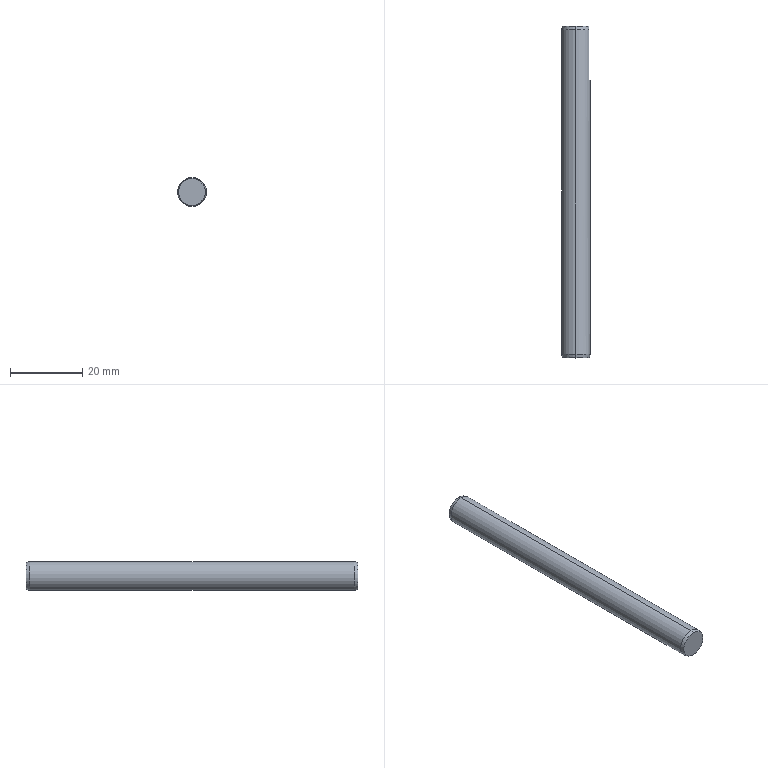Part | SolidWorks | features BaseBody 1 | 1 solid | 11 faces | box 8 x 92 x 8 mm | volume 4599 mm3 | cone 5 | plane 4 | cylinder 2 | commonest cylinder face diameters 8 x2
STEP:
#1=CARTESIAN_POINT('',(3.5,-1.,1.936));
#2=VERTEX_POINT('',#1);
#3=CARTESIAN_POINT('',(0.,-1.,4.));
#4=VERTEX_POINT('',#3);
#5=CARTESIAN_POINT('',(0.,-1.,0.));
#6=DIRECTION('',(0.,-1.,0.));
#7=DIRECTION('',(0.,0.,-1.));
#8=AXIS2_PLACEMENT_3D('',#5,#6,#7);
#9=CIRCLE('',#8,4.);
#10=EDGE_CURVE('',#2,#4,#9,.T.);
#11=ORIENTED_EDGE('',*,*,#10,.T.);
#12=CARTESIAN_POINT('',(0.,-91.,4.));
#13=VERTEX_POINT('',#12);
#14=CARTESIAN_POINT('',(0.,4.6,4.));
#15=DIRECTION('',(0.,-1.,0.));
#16=VECTOR('',#15,1000.);
#17=LINE('',#14,#16);
#18=EDGE_CURVE('',#4,#13,#17,.T.);
#19=ORIENTED_EDGE('',*,*,#18,.T.);
#20=CARTESIAN_POINT('',(0.,-91.,-4.));
#21=VERTEX_POINT('',#20);
#22=CARTESIAN_POINT('',(0.,-91.,0.));
#23=DIRECTION('',(0.,1.,0.));
#24=DIRECTION('',(0.,0.,-1.));
#25=AXIS2_PLACEMENT_3D('',#22,#23,#24);
#26=CIRCLE('',#25,4.);
#27=EDGE_CURVE('',#13,#21,#26,.T.);
#28=ORIENTED_EDGE('',*,*,#27,.T.);
#29=CARTESIAN_POINT('',(0.,-1.,-4.));
#30=VERTEX_POINT('',#29);
#31=CARTESIAN_POINT('',(0.,4.6,-4.));
#32=DIRECTION('',(0.,-1.,0.));
#33=VECTOR('',#32,1000.);
#34=LINE('',#31,#33);
#35=EDGE_CURVE('',#30,#21,#34,.T.);
#36=ORIENTED_EDGE('',*,*,#35,.F.);
#37=CARTESIAN_POINT('',(3.5,-1.,-1.936));
#38=VERTEX_POINT('',#37);
#39=CARTESIAN_POINT('',(0.,-1.,0.));
#40=DIRECTION('',(0.,-1.,0.));
#41=DIRECTION('',(0.,0.,-1.));
#42=AXIS2_PLACEMENT_3D('',#39,#40,#41);
#43=CIRCLE('',#42,4.);
#44=EDGE_CURVE('',#30,#38,#43,.T.);
#45=ORIENTED_EDGE('',*,*,#44,.T.);
#46=CARTESIAN_POINT('',(3.5,-15.,-1.936));
#47=VERTEX_POINT('',#46);
#48=CARTESIAN_POINT('',(3.5,4.6,-1.936));
#49=DIRECTION('',(0.,-1.,0.));
#50=VECTOR('',#49,1000.);
#51=LINE('',#48,#50);
#52=EDGE_CURVE('',#38,#47,#51,.T.);
#53=ORIENTED_EDGE('',*,*,#52,.T.);
#54=CARTESIAN_POINT('',(3.5,-15.,1.936));
#55=VERTEX_POINT('',#54);
#56=CARTESIAN_POINT('',(0.,-15.,0.));
#57=DIRECTION('',(0.,-1.,0.));
#58=DIRECTION('',(0.,0.,-1.));
#59=AXIS2_PLACEMENT_3D('',#56,#57,#58);
#60=CIRCLE('',#59,4.);
#61=EDGE_CURVE('',#47,#55,#60,.T.);
#62=ORIENTED_EDGE('',*,*,#61,.T.);
#63=CARTESIAN_POINT('',(3.5,4.6,1.936));
#64=DIRECTION('',(0.,1.,0.));
#65=VECTOR('',#64,1000.);
#66=LINE('',#63,#65);
#67=EDGE_CURVE('',#55,#2,#66,.T.);
#68=ORIENTED_EDGE('',*,*,#67,.T.);
#69=EDGE_LOOP('',(#11,#19,#28,#36,#45,#53,#62,#68));
#70=FACE_OUTER_BOUND('',#69,.T.);
#71=CARTESIAN_POINT('',(0.,4.6,0.));
#72=DIRECTION('',(0.,-1.,0.));
#73=DIRECTION('',(0.,0.,-1.));
#74=AXIS2_PLACEMENT_3D('',#71,#72,#73);
#75=CYLINDRICAL_SURFACE('',#74,4.);
#76=ADVANCED_FACE('',(#70),#75,.T.);
#77=CARTESIAN_POINT('',(3.5,0.,1.295));
#78=VERTEX_POINT('',#77);
#79=CARTESIAN_POINT('',(0.,0.,3.732));
#80=VERTEX_POINT('',#79);
#81=CARTESIAN_POINT('',(0.,0.,0.));
#82=DIRECTION('',(0.,-1.,0.));
#83=DIRECTION('',(0.,0.,-1.));
#84=AXIS2_PLACEMENT_3D('',#81,#82,#83);
#85=CIRCLE('',#84,3.732);
#86=EDGE_CURVE('',#78,#80,#85,.T.);
#87=ORIENTED_EDGE('',*,*,#86,.T.);
#88=CARTESIAN_POINT('',(0.,-1.,4.));
#89=DIRECTION('',(0.,-0.9659,0.2588));
#90=VECTOR('',#89,1000.);
#91=LINE('',#88,#90);
#92=EDGE_CURVE('',#80,#4,#91,.T.);
#93=ORIENTED_EDGE('',*,*,#92,.T.);
#94=ORIENTED_EDGE('',*,*,#10,.F.);
#95=CARTESIAN_POINT('',(3.5,-1.,1.936));
#96=CARTESIAN_POINT('',(3.5,-0.6058,1.718));
#97=CARTESIAN_POINT('',(3.5,-0.2724,1.506));
#98=CARTESIAN_POINT('',(3.5,0.,1.295));
#99=B_SPLINE_CURVE_WITH_KNOTS('',3,(#95,#96,#97,#98),.UNSPECIFIED.,.F.,.F.,(4,4),(0.,1.),.UNSPECIFIED.);
#100=EDGE_CURVE('',#2,#78,#99,.T.);
#101=ORIENTED_EDGE('',*,*,#100,.T.);
#102=EDGE_LOOP('',(#87,#93,#94,#101));
#103=FACE_OUTER_BOUND('',#102,.T.);
#104=CARTESIAN_POINT('',(0.,-1.,0.));
#105=DIRECTION('',(0.,-1.,0.));
#106=DIRECTION('',(0.,0.,-1.));
#107=AXIS2_PLACEMENT_3D('',#104,#105,#106);
#108=CONICAL_SURFACE('',#107,4.,0.2618);
#109=ADVANCED_FACE('',(#103),#108,.T.);
#110=ORIENTED_EDGE('',*,*,#92,.F.);
#111=CARTESIAN_POINT('',(0.,0.,-3.732));
#112=VERTEX_POINT('',#111);
#113=CARTESIAN_POINT('',(0.,0.,0.));
#114=DIRECTION('',(0.,-1.,0.));
#115=DIRECTION('',(0.,0.,-1.));
#116=AXIS2_PLACEMENT_3D('',#113,#114,#115);
#117=CIRCLE('',#116,3.732);
#118=EDGE_CURVE('',#80,#112,#117,.T.);
#119=ORIENTED_EDGE('',*,*,#118,.T.);
#120=CARTESIAN_POINT('',(0.,-1.,-4.));
#121=DIRECTION('',(0.,-0.9659,-0.2588));
#122=VECTOR('',#121,1000.);
#123=LINE('',#120,#122);
#124=EDGE_CURVE('',#112,#30,#123,.T.);
#125=ORIENTED_EDGE('',*,*,#124,.T.);
#126=CARTESIAN_POINT('',(0.,-1.,0.));
#127=DIRECTION('',(0.,-1.,0.));
#128=DIRECTION('',(0.,0.,-1.));
#129=AXIS2_PLACEMENT_3D('',#126,#127,#128);
#130=CIRCLE('',#129,4.);
#131=EDGE_CURVE('',#4,#30,#130,.T.);
#132=ORIENTED_EDGE('',*,*,#131,.F.);
#133=EDGE_LOOP('',(#110,#119,#125,#132));
#134=FACE_OUTER_BOUND('',#133,.T.);
#135=CARTESIAN_POINT('',(0.,-1.,0.));
#136=DIRECTION('',(0.,-1.,0.));
#137=DIRECTION('',(0.,0.,-1.));
#138=AXIS2_PLACEMENT_3D('',#135,#136,#137);
#139=CONICAL_SURFACE('',#138,4.,0.2618);
#140=ADVANCED_FACE('',(#134),#139,.T.);
#141=CARTESIAN_POINT('',(0.,-92.,3.732));
#142=VERTEX_POINT('',#141);
#143=CARTESIAN_POINT('',(0.,-92.,-3.732));
#144=VERTEX_POINT('',#143);
#145=CARTESIAN_POINT('',(0.,-92.,0.));
#146=DIRECTION('',(0.,1.,0.));
#147=DIRECTION('',(0.,0.,1.));
#148=AXIS2_PLACEMENT_3D('',#145,#146,#147);
#149=CIRCLE('',#148,3.732);
#150=EDGE_CURVE('',#142,#144,#149,.T.);
#151=ORIENTED_EDGE('',*,*,#150,.T.);
#152=CARTESIAN_POINT('',(0.,-91.,-4.));
#153=DIRECTION('',(0.,0.9659,-0.2588));
#154=VECTOR('',#153,1000.);
#155=LINE('',#152,#154);
#156=EDGE_CURVE('',#144,#21,#155,.T.);
#157=ORIENTED_EDGE('',*,*,#156,.T.);
#158=ORIENTED_EDGE('',*,*,#27,.F.);
#159=CARTESIAN_POINT('',(0.,-91.,4.));
#160=DIRECTION('',(0.,0.9659,0.2588));
#161=VECTOR('',#160,1000.);
#162=LINE('',#159,#161);
#163=EDGE_CURVE('',#142,#13,#162,.T.);
#164=ORIENTED_EDGE('',*,*,#163,.F.);
#165=EDGE_LOOP('',(#151,#157,#158,#164));
#166=FACE_OUTER_BOUND('',#165,.T.);
#167=CARTESIAN_POINT('',(0.,-91.,0.));
#168=DIRECTION('',(0.,1.,0.));
#169=DIRECTION('',(0.,0.,1.));
#170=AXIS2_PLACEMENT_3D('',#167,#168,#169);
#171=CONICAL_SURFACE('',#170,4.,0.2618);
#172=ADVANCED_FACE('',(#166),#171,.T.);
#173=ORIENTED_EDGE('',*,*,#150,.F.);
#174=CARTESIAN_POINT('',(0.,-92.,0.));
#175=DIRECTION('',(0.,1.,0.));
#176=DIRECTION('',(0.,0.,1.));
#177=AXIS2_PLACEMENT_3D('',#174,#175,#176);
#178=CIRCLE('',#177,3.732);
#179=EDGE_CURVE('',#144,#142,#178,.T.);
#180=ORIENTED_EDGE('',*,*,#179,.F.);
#181=EDGE_LOOP('',(#173,#180));
#182=FACE_OUTER_BOUND('',#181,.T.);
#183=CARTESIAN_POINT('',(0.,-92.,0.));
#184=DIRECTION('',(0.,-1.,0.));
#185=DIRECTION('',(0.,0.,-1.));
#186=AXIS2_PLACEMENT_3D('',#183,#184,#185);
#187=PLANE('',#186);
#188=ADVANCED_FACE('',(#182),#187,.T.);
#189=ORIENTED_EDGE('',*,*,#86,.F.);
#190=CARTESIAN_POINT('',(3.5,0.,-1.295));
#191=VERTEX_POINT('',#190);
#192=CARTESIAN_POINT('',(3.5,0.,0.));
#193=DIRECTION('',(0.,0.,-1.));
#194=VECTOR('',#193,1000.);
#195=LINE('',#192,#194);
#196=EDGE_CURVE('',#78,#191,#195,.T.);
#197=ORIENTED_EDGE('',*,*,#196,.T.);
#198=CARTESIAN_POINT('',(0.,0.,0.));
#199=DIRECTION('',(0.,-1.,0.));
#200=DIRECTION('',(0.,0.,-1.));
#201=AXIS2_PLACEMENT_3D('',#198,#199,#200);
#202=CIRCLE('',#201,3.732);
#203=EDGE_CURVE('',#112,#191,#202,.T.);
#204=ORIENTED_EDGE('',*,*,#203,.F.);
#205=ORIENTED_EDGE('',*,*,#118,.F.);
#206=EDGE_LOOP('',(#189,#197,#204,#205));
#207=FACE_OUTER_BOUND('',#206,.T.);
#208=CARTESIAN_POINT('',(0.,0.,0.));
#209=DIRECTION('',(0.,-1.,0.));
#210=DIRECTION('',(0.,0.,-1.));
#211=AXIS2_PLACEMENT_3D('',#208,#209,#210);
#212=PLANE('',#211);
#213=ADVANCED_FACE('',(#207),#212,.F.);
#214=CARTESIAN_POINT('',(3.5,-15.,0.));
#215=DIRECTION('',(0.,0.,1.));
#216=VECTOR('',#215,1000.);
#217=LINE('',#214,#216);
#218=EDGE_CURVE('',#47,#55,#217,.T.);
#219=ORIENTED_EDGE('',*,*,#218,.F.);
#220=ORIENTED_EDGE('',*,*,#52,.F.);
#221=CARTESIAN_POINT('',(3.5,0.,-1.295));
#222=CARTESIAN_POINT('',(3.5,-0.2724,-1.506));
#223=CARTESIAN_POINT('',(3.5,-0.6058,-1.718));
#224=CARTESIAN_POINT('',(3.5,-1.,-1.936));
#225=B_SPLINE_CURVE_WITH_KNOTS('',3,(#221,#222,#223,#224),.UNSPECIFIED.,.F.,.F.,(4,4),(0.,1.),.UNSPECIFIED.);
#226=EDGE_CURVE('',#191,#38,#225,.T.);
#227=ORIENTED_EDGE('',*,*,#226,.F.);
#228=ORIENTED_EDGE('',*,*,#196,.F.);
#229=ORIENTED_EDGE('',*,*,#100,.F.);
#230=ORIENTED_EDGE('',*,*,#67,.F.);
#231=EDGE_LOOP('',(#219,#220,#227,#228,#229,#230));
#232=FACE_OUTER_BOUND('',#231,.T.);
#233=CARTESIAN_POINT('',(3.5,0.,0.));
#234=DIRECTION('',(-1.,0.,0.));
#235=DIRECTION('',(0.,0.,1.));
#236=AXIS2_PLACEMENT_3D('',#233,#234,#235);
#237=PLANE('',#236);
#238=ADVANCED_FACE('',(#232),#237,.F.);
#239=ORIENTED_EDGE('',*,*,#218,.T.);
#240=ORIENTED_EDGE('',*,*,#61,.F.);
#241=EDGE_LOOP('',(#239,#240));
#242=FACE_OUTER_BOUND('',#241,.T.);
#243=CARTESIAN_POINT('',(0.,-15.,0.));
#244=DIRECTION('',(0.,1.,0.));
#245=DIRECTION('',(1.,0.,0.));
#246=AXIS2_PLACEMENT_3D('',#243,#244,#245);
#247=PLANE('',#246);
#248=ADVANCED_FACE('',(#242),#247,.T.);
#249=ORIENTED_EDGE('',*,*,#156,.F.);
#250=ORIENTED_EDGE('',*,*,#179,.T.);
#251=ORIENTED_EDGE('',*,*,#163,.T.);
#252=CARTESIAN_POINT('',(0.,-91.,0.));
#253=DIRECTION('',(0.,1.,0.));
#254=DIRECTION('',(0.,0.,-1.));
#255=AXIS2_PLACEMENT_3D('',#252,#253,#254);
#256=CIRCLE('',#255,4.);
#257=EDGE_CURVE('',#21,#13,#256,.T.);
#258=ORIENTED_EDGE('',*,*,#257,.F.);
#259=EDGE_LOOP('',(#249,#250,#251,#258));
#260=FACE_OUTER_BOUND('',#259,.T.);
#261=CARTESIAN_POINT('',(0.,-91.,0.));
#262=DIRECTION('',(0.,1.,0.));
#263=DIRECTION('',(0.,0.,1.));
#264=AXIS2_PLACEMENT_3D('',#261,#262,#263);
#265=CONICAL_SURFACE('',#264,4.,0.2618);
#266=ADVANCED_FACE('',(#260),#265,.T.);
#267=ORIENTED_EDGE('',*,*,#124,.F.);
#268=ORIENTED_EDGE('',*,*,#203,.T.);
#269=ORIENTED_EDGE('',*,*,#226,.T.);
#270=ORIENTED_EDGE('',*,*,#44,.F.);
#271=EDGE_LOOP('',(#267,#268,#269,#270));
#272=FACE_OUTER_BOUND('',#271,.T.);
#273=CARTESIAN_POINT('',(0.,-1.,0.));
#274=DIRECTION('',(0.,-1.,0.));
#275=DIRECTION('',(0.,0.,-1.));
#276=AXIS2_PLACEMENT_3D('',#273,#274,#275);
#277=CONICAL_SURFACE('',#276,4.,0.2618);
#278=ADVANCED_FACE('',(#272),#277,.T.);
#279=ORIENTED_EDGE('',*,*,#18,.F.);
#280=ORIENTED_EDGE('',*,*,#131,.T.);
#281=ORIENTED_EDGE('',*,*,#35,.T.);
#282=ORIENTED_EDGE('',*,*,#257,.T.);
#283=EDGE_LOOP('',(#279,#280,#281,#282));
#284=FACE_OUTER_BOUND('',#283,.T.);
#285=CARTESIAN_POINT('',(0.,4.6,0.));
#286=DIRECTION('',(0.,-1.,0.));
#287=DIRECTION('',(0.,0.,-1.));
#288=AXIS2_PLACEMENT_3D('',#285,#286,#287);
#289=CYLINDRICAL_SURFACE('',#288,4.);
#290=ADVANCED_FACE('',(#284),#289,.T.);
#291=CLOSED_SHELL('',(#76,#109,#140,#172,#188,#213,#238,#248,#266,#278,#290));
#292=MANIFOLD_SOLID_BREP('',#291);
#293=CARTESIAN_POINT('',(0.,0.,0.));
#294=DIRECTION('',(0.,0.,1.));
#295=DIRECTION('',(1.,0.,0.));
#296=AXIS2_PLACEMENT_3D('',#293,#294,#295);
#297=(LENGTH_UNIT()NAMED_UNIT(*)SI_UNIT(.MILLI.,.METRE.));
#298=UNCERTAINTY_MEASURE_WITH_UNIT(LENGTH_MEASURE(0.00001),#297,'','');
#299=(NAMED_UNIT(*)PLANE_ANGLE_UNIT()SI_UNIT($,.RADIAN.));
#300=(NAMED_UNIT(*)SI_UNIT($,.STERADIAN.)SOLID_ANGLE_UNIT());
#301=(GEOMETRIC_REPRESENTATION_CONTEXT(3)GLOBAL_UNCERTAINTY_ASSIGNED_CONTEXT((#298))GLOBAL_UNIT_ASSIGNED_CONTEXT((#297,#299,#300))REPRESENTATION_CONTEXT('',''));
#302=ADVANCED_BREP_SHAPE_REPRESENTATION('',(#292,#296),#301);